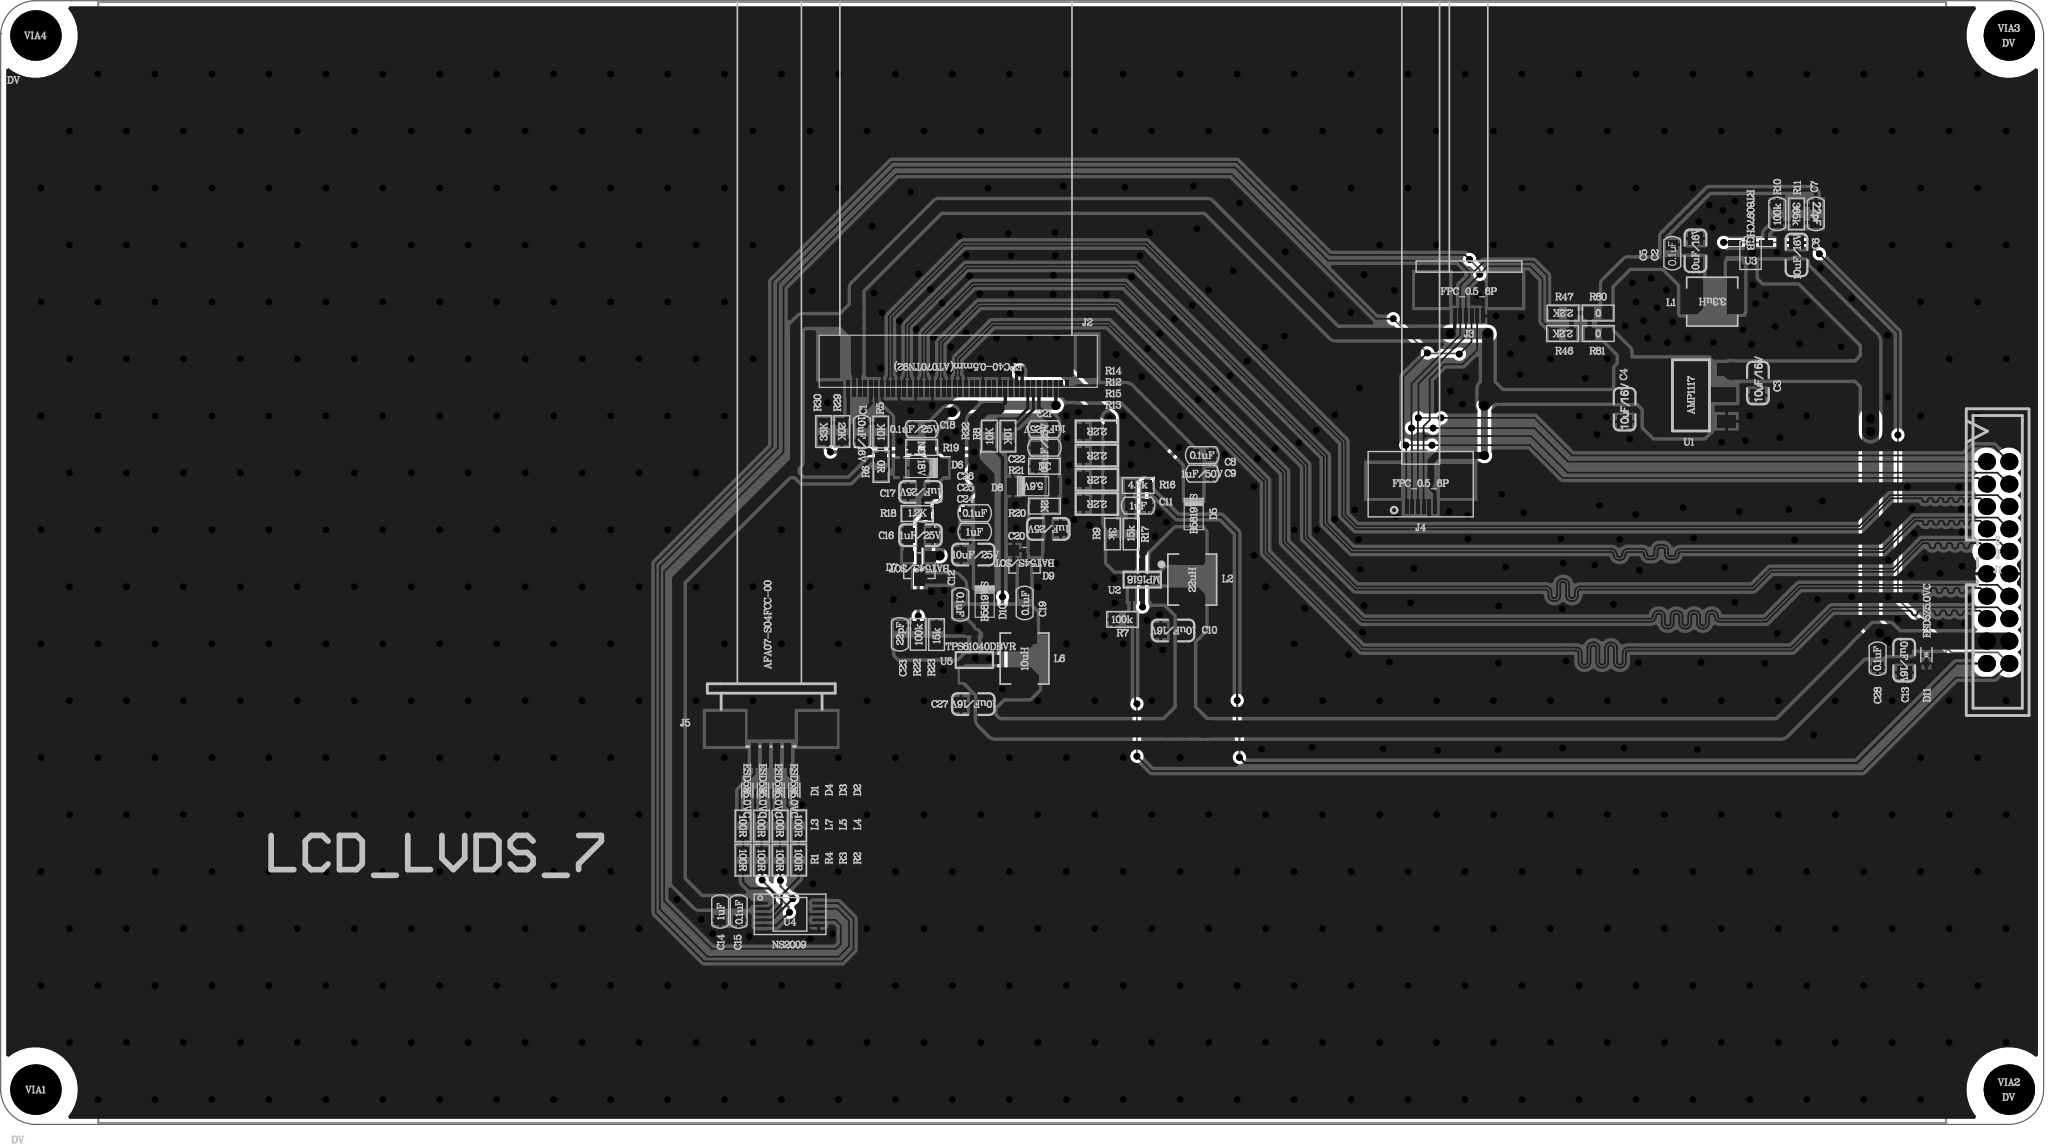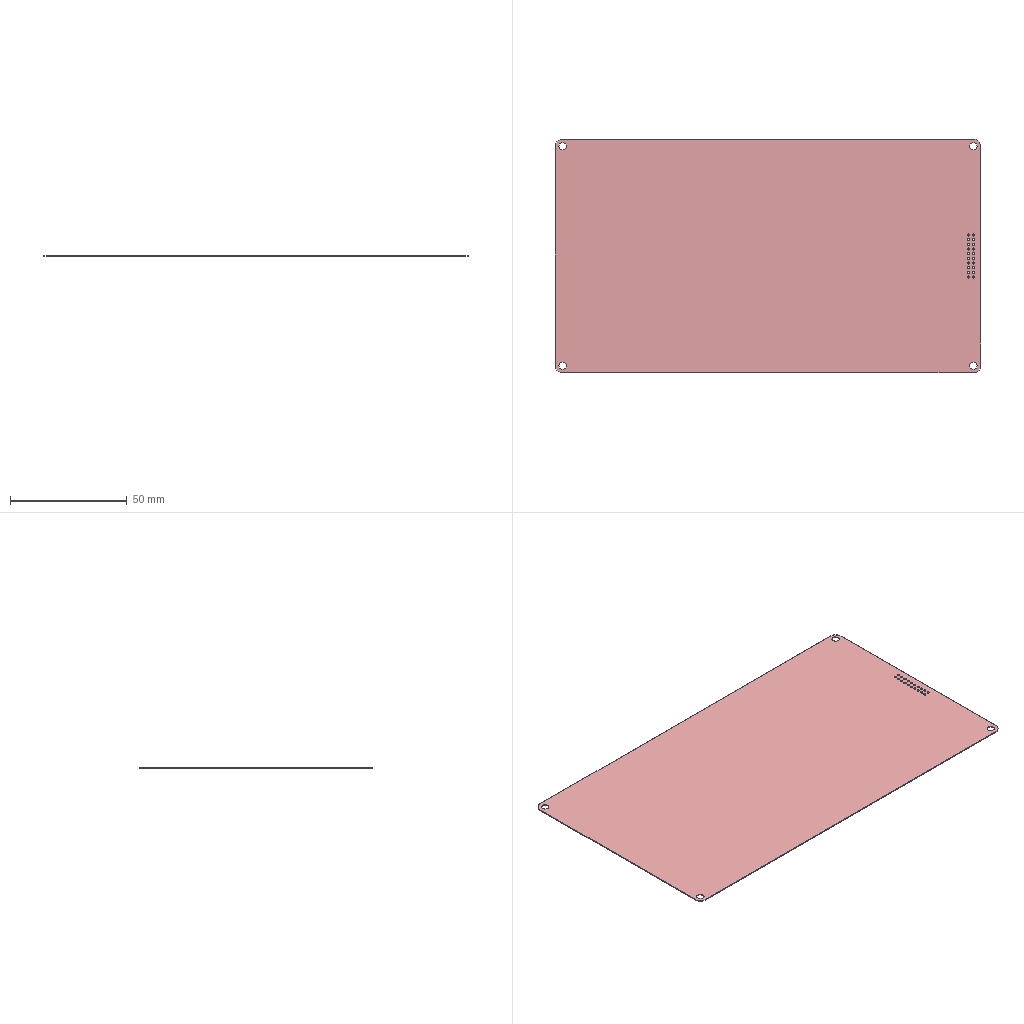Circuit board layout | Altium Designer | box 182.2 x 100.2 x 0.4 mm
Layer stack:
# Altium Designer layer stack of 6 (unit mm; dielectric type: 0 none, 1 core, 2 prepreg, 3 surface material)
index,name,kind,layer,copper_thickness_mm,dielectric_type,dielectric_thickness_mm,dielectric_material,dielectric_constant
0,Paste Mask Top,other,,,,,,
1,Silkscreen Top,other,,,,,,
2,Solder Mask Top,dielectric,,,3,0.0102,Solder Resist,3.5
3,Top,copper,Top,0.0343,,,,
4,Dielectric 1,dielectric,,,0,0.254,FR-4,4.3
5,Bottom,copper,Bottom,0.0343,,,,
6,Solder Mask Bottom,dielectric,,,3,0.0102,Solder Resist,3.5
7,Silkscreen Bottom,other,,,,,,
8,Paste Mask Bottom,other,,,,,,
# drill layer pairs: low layer,high layer
drill_pair,Top,Bottom
Part placement:
Designator,Comment,Layer,Footprint,Center-X(mm),Center-Y(mm),Rotation
D11,ESD5Z5.0VC,TopLayer,SOD-523,171.501,41.758,270
C28,0.1uF,TopLayer,0603C,167.143,41.414,90
C13,10uF/16V,TopLayer,0805C,169.52,41.275,270
VIA4,DV,TopLayer,M3,2.856,96.987,0
VIA3,DV,TopLayer,M3,178.856,96.987,0
VIA2,DV,TopLayer,M3,178.856,2.987,0
VIA1,DV,TopLayer,M3,2.856,2.987,0
C17,1uF/25V,TopLayer,0805C,81.788,56.286,180
D4,ESD5Z5.0VC,TopLayer,SOD-523,67.742,29.667,270
D3,ESD5Z5.0VC,TopLayer,SOD-523,69.139,29.667,270
D2,ESD5Z5.0VC,TopLayer,SOD-523,70.536,29.667,270
D1,ESD5Z5.0VC,TopLayer,SOD-523,66.345,29.667,270
C24,10uF/25V,TopLayer,0805C,86.496,50.7,180
C20,1uF/25V,TopLayer,0805C,93.184,52.986,180
C16,1uF/25V,TopLayer,0805C,81.788,52.426,0
R15,2.2R,TopLayer,0805R,97.52,57.37,180
R14,2.2R,TopLayer,0805R,97.52,61.688,180
R7,100k,TopLayer,0603R,99.805,44.916,0
U5,TPS61040DBVR,TopLayer,SOT-23-5,86.614,41.3,180
R23,15k,TopLayer,0603R,83.22,43.563,270
R22,100k,TopLayer,0603R,81.585,43.586,90
R21,NC,TopLayer,0603R,92.846,58.574,0
R20,2K,TopLayer,0603R,92.846,55.018,0
R19,NC,TopLayer,0603R,81.89,60.249,0
R18,1.2K,TopLayer,0603R,81.483,54.356,0
R17,15k,TopLayer,0603R,100.567,52.536,90
R16,4.7k,TopLayer,0603R,101.202,56.854,0
R9,3k,TopLayer,0603R,98.916,52.536,270
D7,BAT54S/SOT,TopLayer,SOT23,81.686,49.555,180
D6,18V,TopLayer,SOD-123,81.89,58.42,0
C27,10uF/16V,TopLayer,0805C,86.496,37.365,180
C26,0.1uF,TopLayer,0603C,86.623,54.383,180
C25,1uF,TopLayer,0603C,86.623,52.732,180
C23,22pF,TopLayer,0603C,79.959,43.586,270
C22,0.1uF/25V,TopLayer,0603C,92.846,60.225,180
C21,1uF/25V,TopLayer,0603C,92.846,61.876,180
C19,0.1uF,TopLayer,0603C,91.068,46.382,90
C18,0.1uF/25V,TopLayer,0603C,81.89,61.874,180
U4,NS2009,TopLayer,MSOP-10,70.155,18.618,0
R4,100R,TopLayer,0603R,67.615,23.444,270
R3,100R,TopLayer,0603R,69.266,23.444,270
R2,100R,TopLayer,0603R,70.917,23.457,270
R1,100R,TopLayer,0603R,65.964,23.444,270
L7,100R,TopLayer,0603R,67.615,26.492,270
L5,100R,TopLayer,0603R,69.266,26.492,270
L4,100R,TopLayer,0603R,70.917,26.505,270
L3,100R,TopLayer,0603R,65.964,26.492,270
J5,AFA07-S04FCC-00,TopLayer,FPC-SMD-1mm4P-RTP,68.468,33.987,180
C15,0.1uF,TopLayer,0603C,65.583,18.872,270
C14,1uF,TopLayer,0603C,63.932,18.872,270
U3,RT8097CHGB,TopLayer,SOT23-5,155.816,77.572,270
U2,MP1518,TopLayer,SOT-23-6,101.583,48.472,180
U1,AMP1117,TopLayer,SOT223,150.505,64.895,90
R81,0,TopLayer,0603R,142.24,70.409,180
R80,0,TopLayer,0603R,142.224,72.242,0
R8,10K,TopLayer,0603R,89.586,61.263,270
R6,0R,TopLayer,0603R,78.275,58.559,270
R5,10K,TopLayer,0603R,78.25,61.627,90
R47,2.2K,TopLayer,0603R,139.09,72.238,180
R46,2.2K,TopLayer,0603R,139.049,70.413,180
R32,10K,TopLayer,0603R,87.935,61.263,90
R30,33K,TopLayer,0603R,73.152,61.671,90
R29,20K,TopLayer,0603R,74.778,61.671,270
R13,2.2R,TopLayer,0805R,97.52,55.211,180
R12,2.2R,TopLayer,0805R,97.52,59.529,180
R11,365k,TopLayer,0603R,159.918,81.077,270
R10,100k,TopLayer,0603C,158.191,81.077,90
L6,10uH,TopLayer,L-SMD-4*4*1.2,91.068,41.429,90
L2,22uH,TopLayer,L-SMD-4*4*1.2,106.028,48.472,90
L1,3.3uH,TopLayer,L-SMD-4*4*1.2,152.4,73.254,180
J4,FPC_0.5_6P,TopLayer,FPC_0.5_6P_DOWN,126.406,56.137,0
J3,FPC_0.5_6P,TopLayer,FPC_0.5_6P_UP,130.684,73.132,0
J2,FPC40-0.5mm(AT070TN92),TopLayer,FPC40-0.5MM-UP,85.158,66.912,180
J1,DC3-2*10,TopLayer,DC3-2.0-2*10P,177.856,49.987,270
D9,BAT54S/SOT,TopLayer,SOT23,91.068,50.04,180
D8,5.6V,TopLayer,SOD-123,91.83,56.796,180
D5,B5819WS,TopLayer,SOD-123,106.155,54.314,90
D10,B5819WS,TopLayer,SOD-123,87.512,46.509,90
C9,1uF/50V,TopLayer,0603C,106.916,57.926,0
C8,0.1uF,TopLayer,0603C,106.916,59.577,0
C7,22pF,TopLayer,0603C,161.646,81.077,270
C6,10uF/16V,TopLayer,0805C,159.918,77.419,90
C5,0.1uF,TopLayer,0603C,148.831,77.572,90
C4,10uF/16V,TopLayer,0805C,144.589,63.658,270
C3,10uF/16V,TopLayer,0805C,156.476,65.995,270
C2,10uF/16V,TopLayer,0805C,150.908,77.791,90
C12,0.1uF,TopLayer,0603C,85.353,46.255,270
C11,1uF,TopLayer,0603C,101.202,55.076,0
C10,10uF/16V,TopLayer,0805C,104.314,43.927,180
C1,10uF/16V,TopLayer,0603C,76.581,61.638,270
Pad and via stacks:
# Altium Designer via and pad stacks of 6 (unit mm). Each distinct definition once, with the count of objects using it.
# via: kind,start_layer,end_layer,hole_mm,diameter_mm,mode(0 simple;1 top-mid-bottom;2 full stack),diameter_per_layer,count,example_net
# pad: kind,layer,hole_mm,hole_type(0 round;1 square;2 slot),plating,top_size,top_shape(1 round;2 rect;3 octagon;9 rounded rect),mid_size,bottom_size,mode,footprint,size_per_layer,count,example
pad,Top,0,0,plated,1.5x0.3,2,1.5x0.3,1.5x0.3,0,FPC40-0.5MM-UP,,40,J2.1
pad,Top,0,0,plated,3.8x1.8,2,3.8x1.8,3.8x1.8,0,FPC40-0.5MM-UP,,2,J2.41
pad,Top,0,0,plated,1.25x0.3,2,1.25x0.3,1.25x0.3,0,FPC_0.5_6P_UP,,6,J3.1
pad,Top,0,0,plated,3x3,9,3x3,3x3,0,FPC_0.5_6P_UP,,2,J3.7
pad,Top,0,0,plated,1.25x0.3,2,1.25x0.3,1.25x0.3,0,FPC_0.5_6P_DOWN,,6,J4.1
pad,Top,0,0,plated,3x3,9,3x3,3x3,0,FPC_0.5_6P_DOWN,,2,J4.7
pad,Top,0,0,plated,1.4x2.12,2,1.4x2.12,1.4x2.12,0,L-SMD-4*4*1.2,,14,L2.2
pad,Top,0,0,plated,0.85x1,2,0.85x1,0.85x1,0,0603C,,34,C5.1
pad,Top,0,0,plated,1.1x1.27,2,1.1x1.27,1.1x1.27,0,0805C,,20,C3.1
pad,Top,0,0,plated,0.6x0.4,2,0.6x0.4,0.6x0.4,0,SOD-523,,8,D4.2
pad,Top,0,0,plated,0.85x1,2,0.85x1,0.85x1,0,0603R,,50,R7.1
pad,Top,0,0,plated,1.016x1.27,2,1.016x1.27,1.016x1.27,0,0805R,,8,R15.1
pad,Top,0,0,plated,1x1.5,2,1x1.5,1x1.5,0,SOD-123,,8,D6.2
pad,Top,0,0,plated,0.9144x0.9144,2,0.9144x0.9144,0.9144x0.9144,0,SOT23,,4,D7.1
pad,Top,0,0,plated,1.27x0.9144,2,1.27x0.9144,1.27x0.9144,0,SOT23,,2,D7.3
pad,Top,0,0,plated,0.6x1.1,2,0.6x1.1,0.6x1.1,0,SOT-23-5,,3,U5.2
pad,Top,0,0,plated,0.55x1.1,2,0.55x1.1,0.55x1.1,0,SOT-23-5,,2,U5.4
pad,Top,0,0,unplated,1.2x0.25,1,1.2x0.25,1.2x0.25,0,MSOP-10,,10,U4.1
pad,Top,0,0,plated,3.4x3,2,3.4x3,3.4x3,0,FPC-SMD-1mm4P-RTP,,1,J5.6
pad,Top,0,0,plated,3x3.4,2,3x3.4,3x3.4,0,FPC-SMD-1mm4P-RTP,,1,J5.5
pad,Top,0,0,plated,0.6x2.2,2,0.6x2.2,0.6x2.2,0,FPC-SMD-1mm4P-RTP,,4,J5.4
pad,Top,0,0,unplated,1.2x0.5,2,1.2x0.5,1.2x0.5,0,SOT23-5,,5,U3.1
pad,Top,0,0,plated,0.5x1.1,2,0.5x1.1,0.5x1.1,0,SOT-23-6,,6,U2.5
pad,Top,0,0,plated,1.651x1.143,2,1.651x1.143,1.651x1.143,0,SOT223,,3,U1.1
pad,Top,0,0,plated,2.997x1.651,2,2.997x1.651,2.997x1.651,0,SOT223,,1,U1.4
pad,Multi-Layer,0.9144,0,plated,1.524x1.524,1,1.524x1.524,1.524x1.524,0,DC3-2.0-2*10P,,20,J1.1
pad,Multi-Layer,3.2,0,plated,6x6,1,6x6,6x6,0,DV_32_8,,4,VIA4.1
via,Top,Bottom,0.3,0.5,0,,1,
via,Top,Bottom,0.5,1,0,,8,9.3V
Design rules, without the lines most boards share:
# Altium Designer design rules of 6 (exported by Altium Designer, unit mm)
# columns: name | kind | enabled | priority | scope1 | scope2 | descriptor | typed fields (field=value)
POWER | 22 | enabled | 1 | InComponentClass('POWER') | All | Room POWER (Bounding Region = (0mm, 0mm, 50.8mm, 25.4mm) (InComponentClass('POWER')) |
connect | 22 | enabled | 2 | InComponentClass('connect') | All | Room connect (Bounding Region = (0mm, 0mm, 50.8mm, 25.4mm) (InComponentClass('connect')) |
DiffPairsRouting | 51 | enabled | 1 | All | All | Differential Pairs Uncoupled Length using the Gap Constraints (Min=0.254mm) (Max=0.254mm) (Prefered=0.254mm)  and Width Constraints (Min=0.381mm) (Max=0.381mm) (Prefered=0.381mm) (All) |
PlaneClearance | 12 | enabled | 1 | All | All | Power Plane Clearance (Clearance =0.508mm) (All) | clearance=0.508
HoleSize | 42 | enabled | 1 | All | All | Hole Size Constraint (Min=0.025mm) (Max=2.54mm) (All) |
Height | 50 | enabled | 1 | All | All | Height Constraint (Min=0mm) (Max=25.4mm) (Prefered=12.7mm) (All) | min_height=0 max_height=25.4
MinimumSolderMaskSliver | 53 | enabled | 1 | All | All | Minimum Solder Mask Sliver (Gap=0.254mm) (All),(All) |
NetAntennae | 56 | enabled | 1 | All | All | Net Antennae (Tolerance=0mm) (All) |
SilkToSilkClearance | 55 | enabled | 1 | All | All | Silk to Silk (Clearance=0.254mm) (All),(All) |
RoutingCorners | 10 | enabled | 1 | All | All | Routing Corners (Style=45-Degree) (Min Setback=2.54mm) (Max Setback=2.54mm) (All) |
PasteMaskExpansion | 14 | enabled | 1 | All | All | Paste Mask Expansion (Expansion =0mm) (All) | expansion=0
SolderMaskExpansion | 13 | enabled | 1 | All | All | Solder Mask Expansion (Expansion =0.102mm) (All) | expansion=0.1016
ComponentClearance - Default - DEFAULT | 24 | enabled | 1 | All | All | Component Clearance Constraint ( Horizontal Gap = 0.127mm, Vertical Gap = 0.254mm ) (All),(All)  | gap=0.127
Default Width | 2 | enabled | 1 | All | All | Width Constraint (Min=0.15mm) (Max=2mm) (Preferred=0.15mm) (All) |
Default Impedance | 33 | enabled | 1 | All | All | Impedance (Minimum=50.00Ohms Maximum=150.0Ohms) |
Default Parallel Segment Same Layer | 1 | enabled | 2 | All | All | Parallel Segment Constraint (Gap=5.08mm ) (Limit=25.4mm) (All),(All) |
Default Parallel Segment Adjasent | 1 | enabled | 1 | All | All | Parallel Segment Constraint (Gap=5.08mm ) (Limit=25.4mm) (All),(All) |
PolygonConnect - Default Pad | 20 | enabled | 2 | All | All | Polygon Connect Rule(Relief Connect )(Conductor Width=0.2mm) (Relief Angle=45 Angle) (Entries=4) (Air Gap Width=0.254mm) (All),(All) | connect_style(0=relief,1=direct,2=none)=0 relief_conductor_width=0.2 relief_entries=4
Default PlaneConnect | 6 | enabled | 1 | All | All | Power Plane Connect Rule(Relief Connect )(Expansion=0.508mm) (Conductor Width=0.2mm) (Air Gap=0.254mm) (Entries=4) (All) | relief_conductor_width=0.2 relief_entries=4 relief_expansion=0.508
HoleToHoleClearance - Default - DEFAULT | 52 | enabled | 1 | All | All | Hole To Hole Clearance (Gap=0.127mm) (All),(All) | gap=0.127
SMDToCorner - Default - DEFAULT | 23 | enabled | 1 | All | All | SMD To Corner (Distance=0.127mm) (All) |
Clearance - Default - DEFAULT - Net | 0 | enabled | 3 | All | All | Clearance Constraint (Gap=0.15mm) (All),(All) | gap=0.15
RoutingLayers - Default - DEFAULT | 9 | enabled | 1 | All | All | Routing Layers(All) |
Default Length | 3 | enabled | 1 | All | All | Length Constraint (Min=0mm) (Max=1270mm) (All) |
RoutingVias - Default - DEFAULT | 11 | enabled | 1 | All | All | Routing Via (MinHoleWidth=0.3mm) (MaxHoleWidth=0.3mm) (PreferredHoleWidth=0.3mm) (MinWidth=0.6mm) (MaxWidth=0.6mm) (PreferedWidth=0.6mm) (All) | via_min_hole=0.3 via_max_hole=0.3 via_preferred_diameter=0.6 via_preferred_hole=0.3
Default Routing Topology | 7 | enabled | 1 | All | All | Routing Topology Rule(Topology=Shortest) (All) |
RoutingPriority - Default - DEFAULT | 8 | enabled | 1 | All | All | TRoutingPriorityRule(Priority=3) (All) |
Clearance - Default - DEFAULT - Via | 0 | enabled | 2 | IsVia | IsVia | Clearance Constraint (Gap=0.127mm) (IsVia),(IsVia) | gap=0.127
Clearance - Default - DEFAULT- SMD | 0 | enabled | 1 | IsVia | IsSMTPin | Clearance Constraint (Gap=0.127mm) (IsVia),(IsSMTPin) | gap=0.127
PolygonConnect - Default SMT | 20 | enabled | 1 | IsSMTPin | All | Polygon Connect Rule(Relief Connect )(Conductor Width=0.2mm) (Relief Angle=90 Angle) (Entries=4) (Air Gap Width=0.254mm) (IsSMTPin),(All) | connect_style(0=relief,1=direct,2=none)=0 relief_conductor_width=0.2 relief_entries=4
Fanout_SOIC | 49 | enabled | 4 | IsSOIC | All | Fanout Control Rule ( (IsSOIC) ) |
Fanout_Small | 49 | enabled | 3 | (CompPinCount < 5) | All | Fanout Control Rule ( ((CompPinCount < 5)) ) |
SilkToSolderMaskClearance | 54 | enabled | 1 | IsPad | All | Silk To Solder Mask (Clearance=0.254mm) (IsPad),(All) |
Classes set for this board:
# Altium Designer classes of 6 (member kind: 0 net, 1 component, 2 from-to, 3 pad, 4 layer, 5 differential pair, 6 design channel, 7 polygon, 8 structure, 9 xSignal)
# columns: class name | member kind | superclass | members
POWER | 1 | no | C2; C3; C4; C5; C6; C7; C8; C9; C10; C11; C12; D5; D8; D9; D10; L1; L2; L6; R10; R11; R12; R13; TP1; U1; U2; U3; VIA1; VIA2; VIA3; VIA4; C18; C19; C21; C22; C23; C25; C26; C27; D6; D7; R9; R16; R17; R18; R19; R20; R21; R22; R23; U5; R7; R14; R15; C16; C20; C24; C17;
connect | 1 | no | C1; J1; J2; J3; J4; R5; R6; R8; R29; R30; R32; R46; R47; R80; R81; C14; C15; J5; L3; L4; L5; L7; R1; R2; R3; R4; U4; D1; D2; D3; D4;